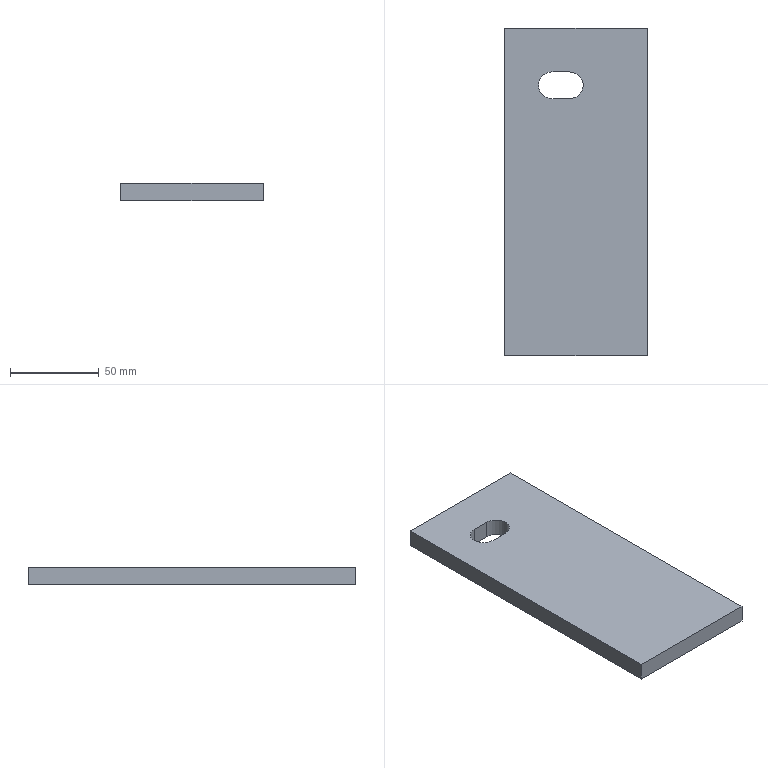Part | STEP file | 计量楼梯支撑Plate | 1 solid | 11 faces | box 80 x 184 x 10 mm | volume 143933 mm3 | plane 8 | cylinder 3 | commonest cylinder face diameters 15 x3
STEP:
#1=CARTESIAN_POINT('',(0.,0.,0.));
#2=DIRECTION('',(0.,0.,1.));
#3=DIRECTION('',(1.,0.,0.));
#4=AXIS2_PLACEMENT_3D('',#1,#2,#3);
#5=CARTESIAN_POINT('',(-13.5,67.5,10.));
#6=VERTEX_POINT('',#5);
#7=CARTESIAN_POINT('',(-13.5,67.5,0.));
#8=VERTEX_POINT('',#7);
#9=CARTESIAN_POINT('',(-13.5,67.5,0.));
#10=DIRECTION('',(0.,0.,-1.));
#11=VECTOR('',#10,1.);
#12=LINE('',#9,#11);
#13=CARTESIAN_POINT('',(-13.5,60.,0.));
#14=DIRECTION('',(0.,0.,-1.));
#15=DIRECTION('',(-1.,0.,0.));
#16=AXIS2_PLACEMENT_3D('',#13,#14,#15);
#17=CYLINDRICAL_SURFACE('',#16,7.5);
#18=CARTESIAN_POINT('',(1.571,0.));
#19=DIRECTION('',(0.,1.));
#20=VECTOR('',#19,1.);
#21=LINE('',#18,#20);
#22=(GEOMETRIC_REPRESENTATION_CONTEXT(2)PARAMETRIC_REPRESENTATION_CONTEXT()REPRESENTATION_CONTEXT('',''));
#23=DEFINITIONAL_REPRESENTATION('',(#21),#22);
#24=PCURVE('',#17,#23);
#25=CARTESIAN_POINT('',(-13.5,67.5,0.));
#26=DIRECTION('',(0.,1.,0.));
#27=DIRECTION('',(0.,0.,1.));
#28=AXIS2_PLACEMENT_3D('',#25,#26,#27);
#29=PLANE('',#28);
#30=CARTESIAN_POINT('',(0.,0.));
#31=DIRECTION('',(-1.,0.));
#32=VECTOR('',#31,1.);
#33=LINE('',#30,#32);
#34=(GEOMETRIC_REPRESENTATION_CONTEXT(2)PARAMETRIC_REPRESENTATION_CONTEXT()REPRESENTATION_CONTEXT('',''));
#35=DEFINITIONAL_REPRESENTATION('',(#33),#34);
#36=PCURVE('',#29,#35);
#37=SURFACE_CURVE('',#12,(#24,#36),.PCURVE_S1.);
#38=EDGE_CURVE('',#6,#8,#37,.T.);
#39=ORIENTED_EDGE('',*,*,#38,.T.);
#40=CARTESIAN_POINT('',(-21.,60.,0.));
#41=VERTEX_POINT('',#40);
#42=CARTESIAN_POINT('',(-13.5,60.,0.));
#43=DIRECTION('',(0.,0.,-1.));
#44=DIRECTION('',(-1.,0.,0.));
#45=AXIS2_PLACEMENT_3D('',#42,#43,#44);
#46=CIRCLE('',#45,7.5);
#47=CARTESIAN_POINT('',(0.,0.));
#48=DIRECTION('',(1.,0.));
#49=VECTOR('',#48,1.);
#50=LINE('',#47,#49);
#51=(GEOMETRIC_REPRESENTATION_CONTEXT(2)PARAMETRIC_REPRESENTATION_CONTEXT()REPRESENTATION_CONTEXT('',''));
#52=DEFINITIONAL_REPRESENTATION('',(#50),#51);
#53=PCURVE('',#17,#52);
#54=CARTESIAN_POINT('',(0.,0.,0.));
#55=DIRECTION('',(0.,0.,1.));
#56=DIRECTION('',(1.,0.,0.));
#57=AXIS2_PLACEMENT_3D('',#54,#55,#56);
#58=PLANE('',#57);
#59=CARTESIAN_POINT('',(-21.,60.));
#60=CARTESIAN_POINT('',(-21.,72.99));
#61=CARTESIAN_POINT('',(-9.75,66.495));
#62=CARTESIAN_POINT('',(1.5,60.));
#63=CARTESIAN_POINT('',(-9.75,53.505));
#64=CARTESIAN_POINT('',(-21.,47.01));
#65=CARTESIAN_POINT('',(-21.,60.));
#66=(BOUNDED_CURVE()B_SPLINE_CURVE(2,(#59,#60,#61,#62,#63,#64,#65),.UNSPECIFIED.,.T.,.F.)B_SPLINE_CURVE_WITH_KNOTS((1,2,2,2,2,1),(-2.094,0.,2.094,4.189,6.283,8.378),.UNSPECIFIED.)CURVE()GEOMETRIC_REPRESENTATION_ITEM()RATIONAL_B_SPLINE_CURVE((1.,0.5,1.,0.5,1.,0.5,1.))REPRESENTATION_ITEM(''));
#67=(GEOMETRIC_REPRESENTATION_CONTEXT(2)PARAMETRIC_REPRESENTATION_CONTEXT()REPRESENTATION_CONTEXT('',''));
#68=DEFINITIONAL_REPRESENTATION('',(#66),#67);
#69=PCURVE('',#58,#68);
#70=SURFACE_CURVE('',#46,(#53,#69),.PCURVE_S1.);
#71=EDGE_CURVE('',#41,#8,#70,.T.);
#72=ORIENTED_EDGE('',*,*,#71,.F.);
#73=CARTESIAN_POINT('',(-21.,60.,10.));
#74=VERTEX_POINT('',#73);
#75=CARTESIAN_POINT('',(-21.,60.,0.));
#76=DIRECTION('',(0.,0.,-1.));
#77=VECTOR('',#76,1.);
#78=LINE('',#75,#77);
#79=CARTESIAN_POINT('',(0.,0.));
#80=DIRECTION('',(0.,1.));
#81=VECTOR('',#80,1.);
#82=LINE('',#79,#81);
#83=(GEOMETRIC_REPRESENTATION_CONTEXT(2)PARAMETRIC_REPRESENTATION_CONTEXT()REPRESENTATION_CONTEXT('',''));
#84=DEFINITIONAL_REPRESENTATION('',(#82),#83);
#85=PCURVE('',#17,#84);
#86=CARTESIAN_POINT('',(-13.5,60.,0.));
#87=DIRECTION('',(0.,0.,-1.));
#88=DIRECTION('',(-1.,0.,0.));
#89=AXIS2_PLACEMENT_3D('',#86,#87,#88);
#90=CYLINDRICAL_SURFACE('',#89,7.5);
#91=CARTESIAN_POINT('',(6.283,0.));
#92=DIRECTION('',(0.,1.));
#93=VECTOR('',#92,1.);
#94=LINE('',#91,#93);
#95=(GEOMETRIC_REPRESENTATION_CONTEXT(2)PARAMETRIC_REPRESENTATION_CONTEXT()REPRESENTATION_CONTEXT('',''));
#96=DEFINITIONAL_REPRESENTATION('',(#94),#95);
#97=PCURVE('',#90,#96);
#98=SURFACE_CURVE('',#78,(#85,#97),.PCURVE_S1.);
#99=EDGE_CURVE('',#74,#41,#98,.T.);
#100=ORIENTED_EDGE('',*,*,#99,.F.);
#101=CARTESIAN_POINT('',(-13.5,60.,10.));
#102=DIRECTION('',(0.,0.,1.));
#103=DIRECTION('',(1.,0.,0.));
#104=AXIS2_PLACEMENT_3D('',#101,#102,#103);
#105=CIRCLE('',#104,7.5);
#106=CARTESIAN_POINT('',(3.142,-10.));
#107=DIRECTION('',(-1.,0.));
#108=VECTOR('',#107,1.);
#109=LINE('',#106,#108);
#110=(GEOMETRIC_REPRESENTATION_CONTEXT(2)PARAMETRIC_REPRESENTATION_CONTEXT()REPRESENTATION_CONTEXT('',''));
#111=DEFINITIONAL_REPRESENTATION('',(#109),#110);
#112=PCURVE('',#17,#111);
#113=CARTESIAN_POINT('',(0.,0.,10.));
#114=DIRECTION('',(0.,0.,1.));
#115=DIRECTION('',(1.,0.,0.));
#116=AXIS2_PLACEMENT_3D('',#113,#114,#115);
#117=PLANE('',#116);
#118=CARTESIAN_POINT('',(-13.5,60.));
#119=DIRECTION('',(1.,0.));
#120=AXIS2_PLACEMENT_2D('',#118,#119);
#121=CIRCLE('',#120,7.5);
#122=(GEOMETRIC_REPRESENTATION_CONTEXT(2)PARAMETRIC_REPRESENTATION_CONTEXT()REPRESENTATION_CONTEXT('',''));
#123=DEFINITIONAL_REPRESENTATION('',(#121),#122);
#124=PCURVE('',#117,#123);
#125=SURFACE_CURVE('',#105,(#112,#124),.PCURVE_S1.);
#126=EDGE_CURVE('',#6,#74,#125,.T.);
#127=ORIENTED_EDGE('',*,*,#126,.F.);
#128=EDGE_LOOP('',(#39,#72,#100,#127));
#129=FACE_BOUND('',#128,.F.);
#130=ADVANCED_FACE('',(#129),#17,.F.);
#131=CARTESIAN_POINT('',(40.,-92.,0.));
#132=VERTEX_POINT('',#131);
#133=CARTESIAN_POINT('',(40.,92.,0.));
#134=VERTEX_POINT('',#133);
#135=CARTESIAN_POINT('',(40.,92.,0.));
#136=DIRECTION('',(0.,1.,0.));
#137=VECTOR('',#136,1.);
#138=LINE('',#135,#137);
#139=CARTESIAN_POINT('',(40.,92.,10.));
#140=DIRECTION('',(-1.,0.,0.));
#141=DIRECTION('',(0.,-1.,0.));
#142=AXIS2_PLACEMENT_3D('',#139,#140,#141);
#143=PLANE('',#142);
#144=CARTESIAN_POINT('',(0.,-10.));
#145=DIRECTION('',(-1.,0.));
#146=VECTOR('',#145,1.);
#147=LINE('',#144,#146);
#148=(GEOMETRIC_REPRESENTATION_CONTEXT(2)PARAMETRIC_REPRESENTATION_CONTEXT()REPRESENTATION_CONTEXT('',''));
#149=DEFINITIONAL_REPRESENTATION('',(#147),#148);
#150=PCURVE('',#143,#149);
#151=CARTESIAN_POINT('',(40.,92.));
#152=DIRECTION('',(0.,1.));
#153=VECTOR('',#152,1.);
#154=LINE('',#151,#153);
#155=(GEOMETRIC_REPRESENTATION_CONTEXT(2)PARAMETRIC_REPRESENTATION_CONTEXT()REPRESENTATION_CONTEXT('',''));
#156=DEFINITIONAL_REPRESENTATION('',(#154),#155);
#157=PCURVE('',#58,#156);
#158=SURFACE_CURVE('',#138,(#150,#157),.PCURVE_S1.);
#159=EDGE_CURVE('',#132,#134,#158,.T.);
#160=ORIENTED_EDGE('',*,*,#159,.T.);
#161=CARTESIAN_POINT('',(40.,92.,10.));
#162=VERTEX_POINT('',#161);
#163=CARTESIAN_POINT('',(40.,92.,10.));
#164=DIRECTION('',(0.,0.,-1.));
#165=VECTOR('',#164,1.);
#166=LINE('',#163,#165);
#167=CARTESIAN_POINT('',(0.,0.));
#168=DIRECTION('',(0.,-1.));
#169=VECTOR('',#168,1.);
#170=LINE('',#167,#169);
#171=(GEOMETRIC_REPRESENTATION_CONTEXT(2)PARAMETRIC_REPRESENTATION_CONTEXT()REPRESENTATION_CONTEXT('',''));
#172=DEFINITIONAL_REPRESENTATION('',(#170),#171);
#173=PCURVE('',#143,#172);
#174=CARTESIAN_POINT('',(-40.,92.,10.));
#175=DIRECTION('',(0.,-1.,0.));
#176=DIRECTION('',(0.,0.,-1.));
#177=AXIS2_PLACEMENT_3D('',#174,#175,#176);
#178=PLANE('',#177);
#179=CARTESIAN_POINT('',(0.,80.));
#180=DIRECTION('',(1.,0.));
#181=VECTOR('',#180,1.);
#182=LINE('',#179,#181);
#183=(GEOMETRIC_REPRESENTATION_CONTEXT(2)PARAMETRIC_REPRESENTATION_CONTEXT()REPRESENTATION_CONTEXT('',''));
#184=DEFINITIONAL_REPRESENTATION('',(#182),#183);
#185=PCURVE('',#178,#184);
#186=SURFACE_CURVE('',#166,(#173,#185),.PCURVE_S1.);
#187=EDGE_CURVE('',#162,#134,#186,.T.);
#188=ORIENTED_EDGE('',*,*,#187,.F.);
#189=CARTESIAN_POINT('',(40.,-92.,10.));
#190=VERTEX_POINT('',#189);
#191=CARTESIAN_POINT('',(40.,92.,10.));
#192=DIRECTION('',(0.,1.,0.));
#193=VECTOR('',#192,1.);
#194=LINE('',#191,#193);
#195=CARTESIAN_POINT('',(0.,0.));
#196=DIRECTION('',(-1.,0.));
#197=VECTOR('',#196,1.);
#198=LINE('',#195,#197);
#199=(GEOMETRIC_REPRESENTATION_CONTEXT(2)PARAMETRIC_REPRESENTATION_CONTEXT()REPRESENTATION_CONTEXT('',''));
#200=DEFINITIONAL_REPRESENTATION('',(#198),#199);
#201=PCURVE('',#143,#200);
#202=CARTESIAN_POINT('',(40.,92.));
#203=DIRECTION('',(0.,1.));
#204=VECTOR('',#203,1.);
#205=LINE('',#202,#204);
#206=(GEOMETRIC_REPRESENTATION_CONTEXT(2)PARAMETRIC_REPRESENTATION_CONTEXT()REPRESENTATION_CONTEXT('',''));
#207=DEFINITIONAL_REPRESENTATION('',(#205),#206);
#208=PCURVE('',#117,#207);
#209=SURFACE_CURVE('',#194,(#201,#208),.PCURVE_S1.);
#210=EDGE_CURVE('',#190,#162,#209,.T.);
#211=ORIENTED_EDGE('',*,*,#210,.F.);
#212=CARTESIAN_POINT('',(40.,-92.,10.));
#213=DIRECTION('',(0.,0.,-1.));
#214=VECTOR('',#213,1.);
#215=LINE('',#212,#214);
#216=CARTESIAN_POINT('',(184.,0.));
#217=DIRECTION('',(0.,-1.));
#218=VECTOR('',#217,1.);
#219=LINE('',#216,#218);
#220=(GEOMETRIC_REPRESENTATION_CONTEXT(2)PARAMETRIC_REPRESENTATION_CONTEXT()REPRESENTATION_CONTEXT('',''));
#221=DEFINITIONAL_REPRESENTATION('',(#219),#220);
#222=PCURVE('',#143,#221);
#223=CARTESIAN_POINT('',(-40.,-92.,10.));
#224=DIRECTION('',(0.,1.,0.));
#225=DIRECTION('',(0.,0.,1.));
#226=AXIS2_PLACEMENT_3D('',#223,#224,#225);
#227=PLANE('',#226);
#228=CARTESIAN_POINT('',(0.,80.));
#229=DIRECTION('',(-1.,0.));
#230=VECTOR('',#229,1.);
#231=LINE('',#228,#230);
#232=(GEOMETRIC_REPRESENTATION_CONTEXT(2)PARAMETRIC_REPRESENTATION_CONTEXT()REPRESENTATION_CONTEXT('',''));
#233=DEFINITIONAL_REPRESENTATION('',(#231),#232);
#234=PCURVE('',#227,#233);
#235=SURFACE_CURVE('',#215,(#222,#234),.PCURVE_S1.);
#236=EDGE_CURVE('',#190,#132,#235,.T.);
#237=ORIENTED_EDGE('',*,*,#236,.T.);
#238=EDGE_LOOP('',(#160,#188,#211,#237));
#239=FACE_BOUND('',#238,.T.);
#240=ADVANCED_FACE('',(#239),#143,.F.);
#241=CARTESIAN_POINT('',(-40.,92.,0.));
#242=VERTEX_POINT('',#241);
#243=CARTESIAN_POINT('',(-40.,92.,0.));
#244=DIRECTION('',(-1.,0.,0.));
#245=VECTOR('',#244,1.);
#246=LINE('',#243,#245);
#247=CARTESIAN_POINT('',(10.,0.));
#248=DIRECTION('',(0.,-1.));
#249=VECTOR('',#248,1.);
#250=LINE('',#247,#249);
#251=(GEOMETRIC_REPRESENTATION_CONTEXT(2)PARAMETRIC_REPRESENTATION_CONTEXT()REPRESENTATION_CONTEXT('',''));
#252=DEFINITIONAL_REPRESENTATION('',(#250),#251);
#253=PCURVE('',#178,#252);
#254=CARTESIAN_POINT('',(-40.,92.));
#255=DIRECTION('',(-1.,0.));
#256=VECTOR('',#255,1.);
#257=LINE('',#254,#256);
#258=(GEOMETRIC_REPRESENTATION_CONTEXT(2)PARAMETRIC_REPRESENTATION_CONTEXT()REPRESENTATION_CONTEXT('',''));
#259=DEFINITIONAL_REPRESENTATION('',(#257),#258);
#260=PCURVE('',#58,#259);
#261=SURFACE_CURVE('',#246,(#253,#260),.PCURVE_S1.);
#262=EDGE_CURVE('',#134,#242,#261,.T.);
#263=ORIENTED_EDGE('',*,*,#262,.T.);
#264=CARTESIAN_POINT('',(-40.,92.,10.));
#265=VERTEX_POINT('',#264);
#266=CARTESIAN_POINT('',(-40.,92.,10.));
#267=DIRECTION('',(0.,0.,-1.));
#268=VECTOR('',#267,1.);
#269=LINE('',#266,#268);
#270=CARTESIAN_POINT('',(0.,0.));
#271=DIRECTION('',(1.,0.));
#272=VECTOR('',#271,1.);
#273=LINE('',#270,#272);
#274=(GEOMETRIC_REPRESENTATION_CONTEXT(2)PARAMETRIC_REPRESENTATION_CONTEXT()REPRESENTATION_CONTEXT('',''));
#275=DEFINITIONAL_REPRESENTATION('',(#273),#274);
#276=PCURVE('',#178,#275);
#277=CARTESIAN_POINT('',(-40.,92.,10.));
#278=DIRECTION('',(1.,0.,0.));
#279=DIRECTION('',(0.,1.,0.));
#280=AXIS2_PLACEMENT_3D('',#277,#278,#279);
#281=PLANE('',#280);
#282=CARTESIAN_POINT('',(0.,0.));
#283=DIRECTION('',(0.,-1.));
#284=VECTOR('',#283,1.);
#285=LINE('',#282,#284);
#286=(GEOMETRIC_REPRESENTATION_CONTEXT(2)PARAMETRIC_REPRESENTATION_CONTEXT()REPRESENTATION_CONTEXT('',''));
#287=DEFINITIONAL_REPRESENTATION('',(#285),#286);
#288=PCURVE('',#281,#287);
#289=SURFACE_CURVE('',#269,(#276,#288),.PCURVE_S1.);
#290=EDGE_CURVE('',#265,#242,#289,.T.);
#291=ORIENTED_EDGE('',*,*,#290,.F.);
#292=CARTESIAN_POINT('',(-40.,92.,10.));
#293=DIRECTION('',(-1.,0.,0.));
#294=VECTOR('',#293,1.);
#295=LINE('',#292,#294);
#296=CARTESIAN_POINT('',(0.,0.));
#297=DIRECTION('',(0.,-1.));
#298=VECTOR('',#297,1.);
#299=LINE('',#296,#298);
#300=(GEOMETRIC_REPRESENTATION_CONTEXT(2)PARAMETRIC_REPRESENTATION_CONTEXT()REPRESENTATION_CONTEXT('',''));
#301=DEFINITIONAL_REPRESENTATION('',(#299),#300);
#302=PCURVE('',#178,#301);
#303=CARTESIAN_POINT('',(-40.,92.));
#304=DIRECTION('',(-1.,0.));
#305=VECTOR('',#304,1.);
#306=LINE('',#303,#305);
#307=(GEOMETRIC_REPRESENTATION_CONTEXT(2)PARAMETRIC_REPRESENTATION_CONTEXT()REPRESENTATION_CONTEXT('',''));
#308=DEFINITIONAL_REPRESENTATION('',(#306),#307);
#309=PCURVE('',#117,#308);
#310=SURFACE_CURVE('',#295,(#302,#309),.PCURVE_S1.);
#311=EDGE_CURVE('',#162,#265,#310,.T.);
#312=ORIENTED_EDGE('',*,*,#311,.F.);
#313=ORIENTED_EDGE('',*,*,#187,.T.);
#314=EDGE_LOOP('',(#263,#291,#312,#313));
#315=FACE_BOUND('',#314,.T.);
#316=ADVANCED_FACE('',(#315),#178,.F.);
#317=CARTESIAN_POINT('',(-40.,-92.,0.));
#318=VERTEX_POINT('',#317);
#319=CARTESIAN_POINT('',(-40.,92.,0.));
#320=DIRECTION('',(0.,-1.,0.));
#321=VECTOR('',#320,1.);
#322=LINE('',#319,#321);
#323=CARTESIAN_POINT('',(0.,-10.));
#324=DIRECTION('',(-1.,0.));
#325=VECTOR('',#324,1.);
#326=LINE('',#323,#325);
#327=(GEOMETRIC_REPRESENTATION_CONTEXT(2)PARAMETRIC_REPRESENTATION_CONTEXT()REPRESENTATION_CONTEXT('',''));
#328=DEFINITIONAL_REPRESENTATION('',(#326),#327);
#329=PCURVE('',#281,#328);
#330=CARTESIAN_POINT('',(-40.,92.));
#331=DIRECTION('',(0.,-1.));
#332=VECTOR('',#331,1.);
#333=LINE('',#330,#332);
#334=(GEOMETRIC_REPRESENTATION_CONTEXT(2)PARAMETRIC_REPRESENTATION_CONTEXT()REPRESENTATION_CONTEXT('',''));
#335=DEFINITIONAL_REPRESENTATION('',(#333),#334);
#336=PCURVE('',#58,#335);
#337=SURFACE_CURVE('',#322,(#329,#336),.PCURVE_S1.);
#338=EDGE_CURVE('',#242,#318,#337,.T.);
#339=ORIENTED_EDGE('',*,*,#338,.T.);
#340=CARTESIAN_POINT('',(-40.,-92.,10.));
#341=VERTEX_POINT('',#340);
#342=CARTESIAN_POINT('',(-40.,-92.,10.));
#343=DIRECTION('',(0.,0.,-1.));
#344=VECTOR('',#343,1.);
#345=LINE('',#342,#344);
#346=CARTESIAN_POINT('',(-184.,0.));
#347=DIRECTION('',(0.,-1.));
#348=VECTOR('',#347,1.);
#349=LINE('',#346,#348);
#350=(GEOMETRIC_REPRESENTATION_CONTEXT(2)PARAMETRIC_REPRESENTATION_CONTEXT()REPRESENTATION_CONTEXT('',''));
#351=DEFINITIONAL_REPRESENTATION('',(#349),#350);
#352=PCURVE('',#281,#351);
#353=CARTESIAN_POINT('',(0.,0.));
#354=DIRECTION('',(-1.,0.));
#355=VECTOR('',#354,1.);
#356=LINE('',#353,#355);
#357=(GEOMETRIC_REPRESENTATION_CONTEXT(2)PARAMETRIC_REPRESENTATION_CONTEXT()REPRESENTATION_CONTEXT('',''));
#358=DEFINITIONAL_REPRESENTATION('',(#356),#357);
#359=PCURVE('',#227,#358);
#360=SURFACE_CURVE('',#345,(#352,#359),.PCURVE_S1.);
#361=EDGE_CURVE('',#341,#318,#360,.T.);
#362=ORIENTED_EDGE('',*,*,#361,.F.);
#363=CARTESIAN_POINT('',(-40.,92.,10.));
#364=DIRECTION('',(0.,-1.,0.));
#365=VECTOR('',#364,1.);
#366=LINE('',#363,#365);
#367=CARTESIAN_POINT('',(0.,0.));
#368=DIRECTION('',(-1.,0.));
#369=VECTOR('',#368,1.);
#370=LINE('',#367,#369);
#371=(GEOMETRIC_REPRESENTATION_CONTEXT(2)PARAMETRIC_REPRESENTATION_CONTEXT()REPRESENTATION_CONTEXT('',''));
#372=DEFINITIONAL_REPRESENTATION('',(#370),#371);
#373=PCURVE('',#281,#372);
#374=CARTESIAN_POINT('',(-40.,92.));
#375=DIRECTION('',(0.,-1.));
#376=VECTOR('',#375,1.);
#377=LINE('',#374,#376);
#378=(GEOMETRIC_REPRESENTATION_CONTEXT(2)PARAMETRIC_REPRESENTATION_CONTEXT()REPRESENTATION_CONTEXT('',''));
#379=DEFINITIONAL_REPRESENTATION('',(#377),#378);
#380=PCURVE('',#117,#379);
#381=SURFACE_CURVE('',#366,(#373,#380),.PCURVE_S1.);
#382=EDGE_CURVE('',#265,#341,#381,.T.);
#383=ORIENTED_EDGE('',*,*,#382,.F.);
#384=ORIENTED_EDGE('',*,*,#290,.T.);
#385=EDGE_LOOP('',(#339,#362,#383,#384));
#386=FACE_BOUND('',#385,.T.);
#387=ADVANCED_FACE('',(#386),#281,.F.);
#388=CARTESIAN_POINT('',(-40.,-92.,0.));
#389=DIRECTION('',(1.,0.,0.));
#390=VECTOR('',#389,1.);
#391=LINE('',#388,#390);
#392=CARTESIAN_POINT('',(-10.,0.));
#393=DIRECTION('',(0.,1.));
#394=VECTOR('',#393,1.);
#395=LINE('',#392,#394);
#396=(GEOMETRIC_REPRESENTATION_CONTEXT(2)PARAMETRIC_REPRESENTATION_CONTEXT()REPRESENTATION_CONTEXT('',''));
#397=DEFINITIONAL_REPRESENTATION('',(#395),#396);
#398=PCURVE('',#227,#397);
#399=CARTESIAN_POINT('',(-40.,-92.));
#400=DIRECTION('',(1.,0.));
#401=VECTOR('',#400,1.);
#402=LINE('',#399,#401);
#403=(GEOMETRIC_REPRESENTATION_CONTEXT(2)PARAMETRIC_REPRESENTATION_CONTEXT()REPRESENTATION_CONTEXT('',''));
#404=DEFINITIONAL_REPRESENTATION('',(#402),#403);
#405=PCURVE('',#58,#404);
#406=SURFACE_CURVE('',#391,(#398,#405),.PCURVE_S1.);
#407=EDGE_CURVE('',#318,#132,#406,.T.);
#408=ORIENTED_EDGE('',*,*,#407,.T.);
#409=ORIENTED_EDGE('',*,*,#236,.F.);
#410=CARTESIAN_POINT('',(-40.,-92.,10.));
#411=DIRECTION('',(1.,0.,0.));
#412=VECTOR('',#411,1.);
#413=LINE('',#410,#412);
#414=CARTESIAN_POINT('',(0.,0.));
#415=DIRECTION('',(0.,1.));
#416=VECTOR('',#415,1.);
#417=LINE('',#414,#416);
#418=(GEOMETRIC_REPRESENTATION_CONTEXT(2)PARAMETRIC_REPRESENTATION_CONTEXT()REPRESENTATION_CONTEXT('',''));
#419=DEFINITIONAL_REPRESENTATION('',(#417),#418);
#420=PCURVE('',#227,#419);
#421=CARTESIAN_POINT('',(-40.,-92.));
#422=DIRECTION('',(1.,0.));
#423=VECTOR('',#422,1.);
#424=LINE('',#421,#423);
#425=(GEOMETRIC_REPRESENTATION_CONTEXT(2)PARAMETRIC_REPRESENTATION_CONTEXT()REPRESENTATION_CONTEXT('',''));
#426=DEFINITIONAL_REPRESENTATION('',(#424),#425);
#427=PCURVE('',#117,#426);
#428=SURFACE_CURVE('',#413,(#420,#427),.PCURVE_S1.);
#429=EDGE_CURVE('',#341,#190,#428,.T.);
#430=ORIENTED_EDGE('',*,*,#429,.F.);
#431=ORIENTED_EDGE('',*,*,#361,.T.);
#432=EDGE_LOOP('',(#408,#409,#430,#431));
#433=FACE_BOUND('',#432,.T.);
#434=ADVANCED_FACE('',(#433),#227,.F.);
#435=CARTESIAN_POINT('',(-13.5,52.5,10.));
#436=VERTEX_POINT('',#435);
#437=CARTESIAN_POINT('',(-3.5,52.5,10.));
#438=VERTEX_POINT('',#437);
#439=CARTESIAN_POINT('',(0.,52.5,10.));
#440=DIRECTION('',(1.,0.,0.));
#441=VECTOR('',#440,1.);
#442=LINE('',#439,#441);
#443=CARTESIAN_POINT('',(0.,52.5));
#444=DIRECTION('',(1.,0.));
#445=VECTOR('',#444,1.);
#446=LINE('',#443,#445);
#447=(GEOMETRIC_REPRESENTATION_CONTEXT(2)PARAMETRIC_REPRESENTATION_CONTEXT()REPRESENTATION_CONTEXT('',''));
#448=DEFINITIONAL_REPRESENTATION('',(#446),#447);
#449=PCURVE('',#117,#448);
#450=CARTESIAN_POINT('',(-13.5,52.5,0.));
#451=DIRECTION('',(0.,-1.,0.));
#452=DIRECTION('',(0.,0.,-1.));
#453=AXIS2_PLACEMENT_3D('',#450,#451,#452);
#454=PLANE('',#453);
#455=CARTESIAN_POINT('',(-10.,13.5));
#456=DIRECTION('',(0.,1.));
#457=VECTOR('',#456,1.);
#458=LINE('',#455,#457);
#459=(GEOMETRIC_REPRESENTATION_CONTEXT(2)PARAMETRIC_REPRESENTATION_CONTEXT()REPRESENTATION_CONTEXT('',''));
#460=DEFINITIONAL_REPRESENTATION('',(#458),#459);
#461=PCURVE('',#454,#460);
#462=SURFACE_CURVE('',#442,(#449,#461),.PCURVE_S1.);
#463=EDGE_CURVE('',#436,#438,#462,.T.);
#464=ORIENTED_EDGE('',*,*,#463,.F.);
#465=CARTESIAN_POINT('',(-13.5,60.,10.));
#466=DIRECTION('',(0.,0.,1.));
#467=DIRECTION('',(1.,0.,0.));
#468=AXIS2_PLACEMENT_3D('',#465,#466,#467);
#469=CIRCLE('',#468,7.5);
#470=CARTESIAN_POINT('',(-13.5,60.));
#471=DIRECTION('',(1.,0.));
#472=AXIS2_PLACEMENT_2D('',#470,#471);
#473=CIRCLE('',#472,7.5);
#474=(GEOMETRIC_REPRESENTATION_CONTEXT(2)PARAMETRIC_REPRESENTATION_CONTEXT()REPRESENTATION_CONTEXT('',''));
#475=DEFINITIONAL_REPRESENTATION('',(#473),#474);
#476=PCURVE('',#117,#475);
#477=CARTESIAN_POINT('',(9.425,-10.));
#478=DIRECTION('',(-1.,0.));
#479=VECTOR('',#478,1.);
#480=LINE('',#477,#479);
#481=(GEOMETRIC_REPRESENTATION_CONTEXT(2)PARAMETRIC_REPRESENTATION_CONTEXT()REPRESENTATION_CONTEXT('',''));
#482=DEFINITIONAL_REPRESENTATION('',(#480),#481);
#483=PCURVE('',#90,#482);
#484=SURFACE_CURVE('',#469,(#476,#483),.PCURVE_S1.);
#485=EDGE_CURVE('',#74,#436,#484,.T.);
#486=ORIENTED_EDGE('',*,*,#485,.F.);
#487=ORIENTED_EDGE('',*,*,#126,.F.);
#488=CARTESIAN_POINT('',(-3.5,67.5,10.));
#489=VERTEX_POINT('',#488);
#490=CARTESIAN_POINT('',(0.,67.5,10.));
#491=DIRECTION('',(-1.,0.,0.));
#492=VECTOR('',#491,1.);
#493=LINE('',#490,#492);
#494=CARTESIAN_POINT('',(0.,67.5));
#495=DIRECTION('',(-1.,0.));
#496=VECTOR('',#495,1.);
#497=LINE('',#494,#496);
#498=(GEOMETRIC_REPRESENTATION_CONTEXT(2)PARAMETRIC_REPRESENTATION_CONTEXT()REPRESENTATION_CONTEXT('',''));
#499=DEFINITIONAL_REPRESENTATION('',(#497),#498);
#500=PCURVE('',#117,#499);
#501=CARTESIAN_POINT('',(10.,13.5));
#502=DIRECTION('',(0.,-1.));
#503=VECTOR('',#502,1.);
#504=LINE('',#501,#503);
#505=(GEOMETRIC_REPRESENTATION_CONTEXT(2)PARAMETRIC_REPRESENTATION_CONTEXT()REPRESENTATION_CONTEXT('',''));
#506=DEFINITIONAL_REPRESENTATION('',(#504),#505);
#507=PCURVE('',#29,#506);
#508=SURFACE_CURVE('',#493,(#500,#507),.PCURVE_S1.);
#509=EDGE_CURVE('',#489,#6,#508,.T.);
#510=ORIENTED_EDGE('',*,*,#509,.F.);
#511=CARTESIAN_POINT('',(-3.5,60.,10.));
#512=DIRECTION('',(0.,0.,1.));
#513=DIRECTION('',(1.,0.,0.));
#514=AXIS2_PLACEMENT_3D('',#511,#512,#513);
#515=CIRCLE('',#514,7.5);
#516=CARTESIAN_POINT('',(-3.5,60.));
#517=DIRECTION('',(1.,0.));
#518=AXIS2_PLACEMENT_2D('',#516,#517);
#519=CIRCLE('',#518,7.5);
#520=(GEOMETRIC_REPRESENTATION_CONTEXT(2)PARAMETRIC_REPRESENTATION_CONTEXT()REPRESENTATION_CONTEXT('',''));
#521=DEFINITIONAL_REPRESENTATION('',(#519),#520);
#522=PCURVE('',#117,#521);
#523=CARTESIAN_POINT('',(-3.5,60.,0.));
#524=DIRECTION('',(0.,0.,-1.));
#525=DIRECTION('',(-1.,0.,0.));
#526=AXIS2_PLACEMENT_3D('',#523,#524,#525);
#527=CYLINDRICAL_SURFACE('',#526,7.5);
#528=CARTESIAN_POINT('',(9.425,-10.));
#529=DIRECTION('',(-1.,0.));
#530=VECTOR('',#529,1.);
#531=LINE('',#528,#530);
#532=(GEOMETRIC_REPRESENTATION_CONTEXT(2)PARAMETRIC_REPRESENTATION_CONTEXT()REPRESENTATION_CONTEXT('',''));
#533=DEFINITIONAL_REPRESENTATION('',(#531),#532);
#534=PCURVE('',#527,#533);
#535=SURFACE_CURVE('',#515,(#522,#534),.PCURVE_S1.);
#536=EDGE_CURVE('',#438,#489,#535,.T.);
#537=ORIENTED_EDGE('',*,*,#536,.F.);
#538=EDGE_LOOP('',(#464,#486,#487,#510,#537));
#539=FACE_BOUND('',#538,.T.);
#540=ORIENTED_EDGE('',*,*,#210,.T.);
#541=ORIENTED_EDGE('',*,*,#311,.T.);
#542=ORIENTED_EDGE('',*,*,#382,.T.);
#543=ORIENTED_EDGE('',*,*,#429,.T.);
#544=EDGE_LOOP('',(#540,#541,#542,#543));
#545=FACE_BOUND('',#544,.T.);
#546=ADVANCED_FACE('',(#539,#545),#117,.T.);
#547=CARTESIAN_POINT('',(-3.5,67.5,0.));
#548=VERTEX_POINT('',#547);
#549=CARTESIAN_POINT('',(-3.5,52.5,0.));
#550=VERTEX_POINT('',#549);
#551=CARTESIAN_POINT('',(-3.5,60.,0.));
#552=DIRECTION('',(0.,0.,-1.));
#553=DIRECTION('',(-1.,0.,0.));
#554=AXIS2_PLACEMENT_3D('',#551,#552,#553);
#555=CIRCLE('',#554,7.5);
#556=CARTESIAN_POINT('',(-11.,60.));
#557=CARTESIAN_POINT('',(-11.,72.99));
#558=CARTESIAN_POINT('',(0.25,66.495));
#559=CARTESIAN_POINT('',(11.5,60.));
#560=CARTESIAN_POINT('',(0.25,53.505));
#561=CARTESIAN_POINT('',(-11.,47.01));
#562=CARTESIAN_POINT('',(-11.,60.));
#563=(BOUNDED_CURVE()B_SPLINE_CURVE(2,(#556,#557,#558,#559,#560,#561,#562),.UNSPECIFIED.,.T.,.F.)B_SPLINE_CURVE_WITH_KNOTS((1,2,2,2,2,1),(-2.094,0.,2.094,4.189,6.283,8.378),.UNSPECIFIED.)CURVE()GEOMETRIC_REPRESENTATION_ITEM()RATIONAL_B_SPLINE_CURVE((1.,0.5,1.,0.5,1.,0.5,1.))REPRESENTATION_ITEM(''));
#564=(GEOMETRIC_REPRESENTATION_CONTEXT(2)PARAMETRIC_REPRESENTATION_CONTEXT()REPRESENTATION_CONTEXT('',''));
#565=DEFINITIONAL_REPRESENTATION('',(#563),#564);
#566=PCURVE('',#58,#565);
#567=CARTESIAN_POINT('',(0.,0.));
#568=DIRECTION('',(1.,0.));
#569=VECTOR('',#568,1.);
#570=LINE('',#567,#569);
#571=(GEOMETRIC_REPRESENTATION_CONTEXT(2)PARAMETRIC_REPRESENTATION_CONTEXT()REPRESENTATION_CONTEXT('',''));
#572=DEFINITIONAL_REPRESENTATION('',(#570),#571);
#573=PCURVE('',#527,#572);
#574=SURFACE_CURVE('',#555,(#566,#573),.PCURVE_S1.);
#575=EDGE_CURVE('',#548,#550,#574,.T.);
#576=ORIENTED_EDGE('',*,*,#575,.F.);
#577=CARTESIAN_POINT('',(-13.5,67.5,0.));
#578=DIRECTION('',(1.,0.,0.));
#579=VECTOR('',#578,1.);
#580=LINE('',#577,#579);
#581=CARTESIAN_POINT('',(-13.5,67.5));
#582=DIRECTION('',(1.,0.));
#583=VECTOR('',#582,1.);
#584=LINE('',#581,#583);
#585=(GEOMETRIC_REPRESENTATION_CONTEXT(2)PARAMETRIC_REPRESENTATION_CONTEXT()REPRESENTATION_CONTEXT('',''));
#586=DEFINITIONAL_REPRESENTATION('',(#584),#585);
#587=PCURVE('',#58,#586);
#588=CARTESIAN_POINT('',(0.,0.));
#589=DIRECTION('',(0.,1.));
#590=VECTOR('',#589,1.);
#591=LINE('',#588,#590);
#592=(GEOMETRIC_REPRESENTATION_CONTEXT(2)PARAMETRIC_REPRESENTATION_CONTEXT()REPRESENTATION_CONTEXT('',''));
#593=DEFINITIONAL_REPRESENTATION('',(#591),#592);
#594=PCURVE('',#29,#593);
#595=SURFACE_CURVE('',#580,(#587,#594),.PCURVE_S1.);
#596=EDGE_CURVE('',#8,#548,#595,.T.);
#597=ORIENTED_EDGE('',*,*,#596,.F.);
#598=ORIENTED_EDGE('',*,*,#71,.F.);
#599=CARTESIAN_POINT('',(-13.5,52.5,0.));
#600=VERTEX_POINT('',#599);
#601=CARTESIAN_POINT('',(-13.5,60.,0.));
#602=DIRECTION('',(0.,0.,-1.));
#603=DIRECTION('',(-1.,0.,0.));
#604=AXIS2_PLACEMENT_3D('',#601,#602,#603);
#605=CIRCLE('',#604,7.5);
#606=CARTESIAN_POINT('',(-21.,60.));
#607=CARTESIAN_POINT('',(-21.,72.99));
#608=CARTESIAN_POINT('',(-9.75,66.495));
#609=CARTESIAN_POINT('',(1.5,60.));
#610=CARTESIAN_POINT('',(-9.75,53.505));
#611=CARTESIAN_POINT('',(-21.,47.01));
#612=CARTESIAN_POINT('',(-21.,60.));
#613=(BOUNDED_CURVE()B_SPLINE_CURVE(2,(#606,#607,#608,#609,#610,#611,#612),.UNSPECIFIED.,.T.,.F.)B_SPLINE_CURVE_WITH_KNOTS((1,2,2,2,2,1),(-2.094,0.,2.094,4.189,6.283,8.378),.UNSPECIFIED.)CURVE()GEOMETRIC_REPRESENTATION_ITEM()RATIONAL_B_SPLINE_CURVE((1.,0.5,1.,0.5,1.,0.5,1.))REPRESENTATION_ITEM(''));
#614=(GEOMETRIC_REPRESENTATION_CONTEXT(2)PARAMETRIC_REPRESENTATION_CONTEXT()REPRESENTATION_CONTEXT('',''));
#615=DEFINITIONAL_REPRESENTATION('',(#613),#614);
#616=PCURVE('',#58,#615);
#617=CARTESIAN_POINT('',(0.,0.));
#618=DIRECTION('',(1.,0.));
#619=VECTOR('',#618,1.);
#620=LINE('',#617,#619);
#621=(GEOMETRIC_REPRESENTATION_CONTEXT(2)PARAMETRIC_REPRESENTATION_CONTEXT()REPRESENTATION_CONTEXT('',''));
#622=DEFINITIONAL_REPRESENTATION('',(#620),#621);
#623=PCURVE('',#90,#622);
#624=SURFACE_CURVE('',#605,(#616,#623),.PCURVE_S1.);
#625=EDGE_CURVE('',#600,#41,#624,.T.);
#626=ORIENTED_EDGE('',*,*,#625,.F.);
#627=CARTESIAN_POINT('',(-13.5,52.5,0.));
#628=DIRECTION('',(1.,0.,0.));
#629=VECTOR('',#628,1.);
#630=LINE('',#627,#629);
#631=CARTESIAN_POINT('',(-13.5,52.5));
#632=DIRECTION('',(1.,0.));
#633=VECTOR('',#632,1.);
#634=LINE('',#631,#633);
#635=(GEOMETRIC_REPRESENTATION_CONTEXT(2)PARAMETRIC_REPRESENTATION_CONTEXT()REPRESENTATION_CONTEXT('',''));
#636=DEFINITIONAL_REPRESENTATION('',(#634),#635);
#637=PCURVE('',#58,#636);
#638=CARTESIAN_POINT('',(0.,0.));
#639=DIRECTION('',(0.,1.));
#640=VECTOR('',#639,1.);
#641=LINE('',#638,#640);
#642=(GEOMETRIC_REPRESENTATION_CONTEXT(2)PARAMETRIC_REPRESENTATION_CONTEXT()REPRESENTATION_CONTEXT('',''));
#643=DEFINITIONAL_REPRESENTATION('',(#641),#642);
#644=PCURVE('',#454,#643);
#645=SURFACE_CURVE('',#630,(#637,#644),.PCURVE_S1.);
#646=EDGE_CURVE('',#600,#550,#645,.T.);
#647=ORIENTED_EDGE('',*,*,#646,.T.);
#648=EDGE_LOOP('',(#576,#597,#598,#626,#647));
#649=FACE_BOUND('',#648,.T.);
#650=ORIENTED_EDGE('',*,*,#159,.F.);
#651=ORIENTED_EDGE('',*,*,#407,.F.);
#652=ORIENTED_EDGE('',*,*,#338,.F.);
#653=ORIENTED_EDGE('',*,*,#262,.F.);
#654=EDGE_LOOP('',(#650,#651,#652,#653));
#655=FACE_BOUND('',#654,.T.);
#656=ADVANCED_FACE('',(#649,#655),#58,.F.);
#657=CARTESIAN_POINT('',(-3.5,52.5,0.));
#658=DIRECTION('',(0.,0.,-1.));
#659=VECTOR('',#658,1.);
#660=LINE('',#657,#659);
#661=CARTESIAN_POINT('',(4.712,0.));
#662=DIRECTION('',(0.,1.));
#663=VECTOR('',#662,1.);
#664=LINE('',#661,#663);
#665=(GEOMETRIC_REPRESENTATION_CONTEXT(2)PARAMETRIC_REPRESENTATION_CONTEXT()REPRESENTATION_CONTEXT('',''));
#666=DEFINITIONAL_REPRESENTATION('',(#664),#665);
#667=PCURVE('',#527,#666);
#668=CARTESIAN_POINT('',(0.,10.));
#669=DIRECTION('',(1.,0.));
#670=VECTOR('',#669,1.);
#671=LINE('',#668,#670);
#672=(GEOMETRIC_REPRESENTATION_CONTEXT(2)PARAMETRIC_REPRESENTATION_CONTEXT()REPRESENTATION_CONTEXT('',''));
#673=DEFINITIONAL_REPRESENTATION('',(#671),#672);
#674=PCURVE('',#454,#673);
#675=SURFACE_CURVE('',#660,(#667,#674),.PCURVE_S1.);
#676=EDGE_CURVE('',#438,#550,#675,.T.);
#677=ORIENTED_EDGE('',*,*,#676,.T.);
#678=ORIENTED_EDGE('',*,*,#575,.F.);
#679=CARTESIAN_POINT('',(-3.5,67.5,0.));
#680=DIRECTION('',(0.,0.,1.));
#681=VECTOR('',#680,1.);
#682=LINE('',#679,#681);
#683=CARTESIAN_POINT('',(1.571,0.));
#684=DIRECTION('',(0.,-1.));
#685=VECTOR('',#684,1.);
#686=LINE('',#683,#685);
#687=(GEOMETRIC_REPRESENTATION_CONTEXT(2)PARAMETRIC_REPRESENTATION_CONTEXT()REPRESENTATION_CONTEXT('',''));
#688=DEFINITIONAL_REPRESENTATION('',(#686),#687);
#689=PCURVE('',#527,#688);
#690=CARTESIAN_POINT('',(0.,10.));
#691=DIRECTION('',(1.,0.));
#692=VECTOR('',#691,1.);
#693=LINE('',#690,#692);
#694=(GEOMETRIC_REPRESENTATION_CONTEXT(2)PARAMETRIC_REPRESENTATION_CONTEXT()REPRESENTATION_CONTEXT('',''));
#695=DEFINITIONAL_REPRESENTATION('',(#693),#694);
#696=PCURVE('',#29,#695);
#697=SURFACE_CURVE('',#682,(#689,#696),.PCURVE_S1.);
#698=EDGE_CURVE('',#548,#489,#697,.T.);
#699=ORIENTED_EDGE('',*,*,#698,.T.);
#700=ORIENTED_EDGE('',*,*,#536,.F.);
#701=EDGE_LOOP('',(#677,#678,#699,#700));
#702=FACE_BOUND('',#701,.F.);
#703=ADVANCED_FACE('',(#702),#527,.F.);
#704=ORIENTED_EDGE('',*,*,#625,.F.);
#705=CARTESIAN_POINT('',(-13.5,52.5,0.));
#706=DIRECTION('',(0.,0.,1.));
#707=VECTOR('',#706,1.);
#708=LINE('',#705,#707);
#709=CARTESIAN_POINT('',(4.712,0.));
#710=DIRECTION('',(0.,-1.));
#711=VECTOR('',#710,1.);
#712=LINE('',#709,#711);
#713=(GEOMETRIC_REPRESENTATION_CONTEXT(2)PARAMETRIC_REPRESENTATION_CONTEXT()REPRESENTATION_CONTEXT('',''));
#714=DEFINITIONAL_REPRESENTATION('',(#712),#713);
#715=PCURVE('',#90,#714);
#716=CARTESIAN_POINT('',(0.,0.));
#717=DIRECTION('',(-1.,0.));
#718=VECTOR('',#717,1.);
#719=LINE('',#716,#718);
#720=(GEOMETRIC_REPRESENTATION_CONTEXT(2)PARAMETRIC_REPRESENTATION_CONTEXT()REPRESENTATION_CONTEXT('',''));
#721=DEFINITIONAL_REPRESENTATION('',(#719),#720);
#722=PCURVE('',#454,#721);
#723=SURFACE_CURVE('',#708,(#715,#722),.PCURVE_S1.);
#724=EDGE_CURVE('',#600,#436,#723,.T.);
#725=ORIENTED_EDGE('',*,*,#724,.T.);
#726=ORIENTED_EDGE('',*,*,#485,.F.);
#727=ORIENTED_EDGE('',*,*,#99,.T.);
#728=EDGE_LOOP('',(#704,#725,#726,#727));
#729=FACE_BOUND('',#728,.F.);
#730=ADVANCED_FACE('',(#729),#90,.F.);
#731=ORIENTED_EDGE('',*,*,#463,.T.);
#732=ORIENTED_EDGE('',*,*,#676,.T.);
#733=ORIENTED_EDGE('',*,*,#646,.F.);
#734=ORIENTED_EDGE('',*,*,#724,.T.);
#735=EDGE_LOOP('',(#731,#732,#733,#734));
#736=FACE_BOUND('',#735,.T.);
#737=ADVANCED_FACE('',(#736),#454,.F.);
#738=ORIENTED_EDGE('',*,*,#509,.T.);
#739=ORIENTED_EDGE('',*,*,#38,.T.);
#740=ORIENTED_EDGE('',*,*,#596,.T.);
#741=ORIENTED_EDGE('',*,*,#698,.T.);
#742=EDGE_LOOP('',(#738,#739,#740,#741));
#743=FACE_BOUND('',#742,.T.);
#744=ADVANCED_FACE('',(#743),#29,.F.);
#745=CLOSED_SHELL('',(#130,#240,#316,#387,#434,#546,#656,#703,#730,#737,#744));
#746=MANIFOLD_SOLID_BREP('',#745);
#747=(LENGTH_UNIT()NAMED_UNIT(*)SI_UNIT(.MILLI.,.METRE.));
#748=UNCERTAINTY_MEASURE_WITH_UNIT(LENGTH_MEASURE(0.0000001),#747,'','');
#749=(NAMED_UNIT(*)PLANE_ANGLE_UNIT()SI_UNIT($,.RADIAN.));
#750=(NAMED_UNIT(*)SI_UNIT($,.STERADIAN.)SOLID_ANGLE_UNIT());
#751=(GEOMETRIC_REPRESENTATION_CONTEXT(3)GLOBAL_UNCERTAINTY_ASSIGNED_CONTEXT((#748))GLOBAL_UNIT_ASSIGNED_CONTEXT((#747,#749,#750))REPRESENTATION_CONTEXT('',''));
#752=ADVANCED_BREP_SHAPE_REPRESENTATION('',(#4,#746),#751);